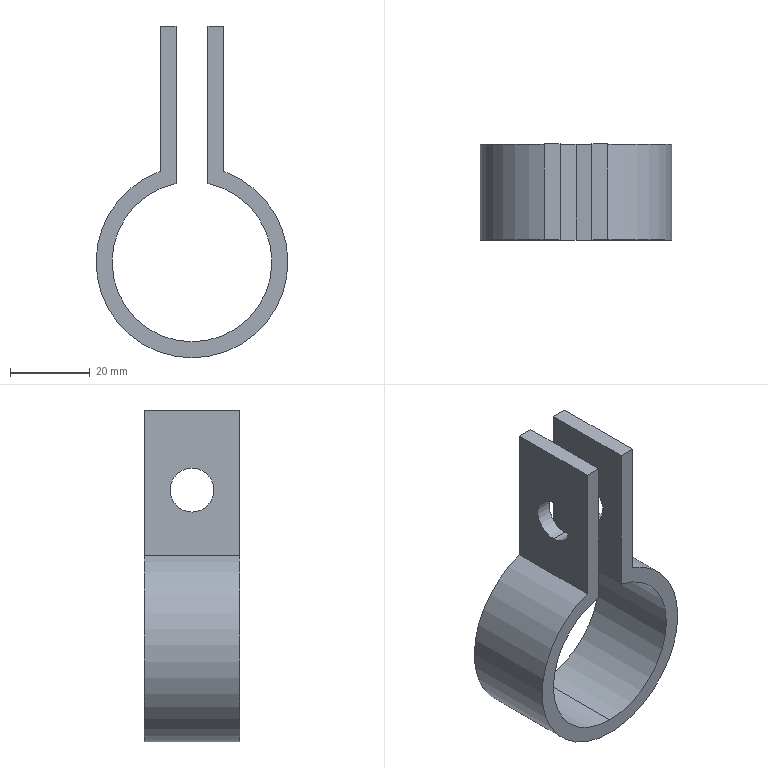Part | SolidWorks | features Extrusion 1, ICE 1 | 1 solid | 16 faces | box 48 x 24 x 83 mm | volume 18610 mm3 | cylinder 8 | plane 8 | commonest cylinder face diameters 11 x4 40 x2 48 x2
STEP:
#1=CARTESIAN_POINT('',(-8.,0.,44.5));
#2=VERTEX_POINT('',#1);
#3=CARTESIAN_POINT('',(-8.,0.,33.5));
#4=VERTEX_POINT('',#3);
#5=CARTESIAN_POINT('',(-8.,0.,39.));
#6=DIRECTION('',(1.,0.,0.));
#7=DIRECTION('',(0.,0.,-1.));
#8=AXIS2_PLACEMENT_3D('',#5,#6,#7);
#9=CIRCLE('',#8,5.5);
#10=EDGE_CURVE('',#2,#4,#9,.T.);
#11=ORIENTED_EDGE('',*,*,#10,.F.);
#12=CARTESIAN_POINT('',(-4.,0.,44.5));
#13=VERTEX_POINT('',#12);
#14=CARTESIAN_POINT('',(-24.,0.,44.5));
#15=DIRECTION('',(1.,0.,0.));
#16=VECTOR('',#15,1000.);
#17=LINE('',#14,#16);
#18=EDGE_CURVE('',#2,#13,#17,.T.);
#19=ORIENTED_EDGE('',*,*,#18,.T.);
#20=CARTESIAN_POINT('',(-4.,0.,33.5));
#21=VERTEX_POINT('',#20);
#22=CARTESIAN_POINT('',(-4.,0.,39.));
#23=DIRECTION('',(-1.,0.,0.));
#24=DIRECTION('',(0.,0.,1.));
#25=AXIS2_PLACEMENT_3D('',#22,#23,#24);
#26=CIRCLE('',#25,5.5);
#27=EDGE_CURVE('',#21,#13,#26,.T.);
#28=ORIENTED_EDGE('',*,*,#27,.F.);
#29=CARTESIAN_POINT('',(-24.,0.,33.5));
#30=DIRECTION('',(1.,0.,0.));
#31=VECTOR('',#30,1000.);
#32=LINE('',#29,#31);
#33=EDGE_CURVE('',#4,#21,#32,.T.);
#34=ORIENTED_EDGE('',*,*,#33,.F.);
#35=EDGE_LOOP('',(#11,#19,#28,#34));
#36=FACE_OUTER_BOUND('',#35,.T.);
#37=CARTESIAN_POINT('',(-24.,0.,39.));
#38=DIRECTION('',(1.,0.,0.));
#39=DIRECTION('',(0.,0.,-1.));
#40=AXIS2_PLACEMENT_3D('',#37,#38,#39);
#41=CYLINDRICAL_SURFACE('',#40,5.5);
#42=ADVANCED_FACE('',(#36),#41,.F.);
#43=CARTESIAN_POINT('',(4.,0.,44.5));
#44=VERTEX_POINT('',#43);
#45=CARTESIAN_POINT('',(4.,0.,33.5));
#46=VERTEX_POINT('',#45);
#47=CARTESIAN_POINT('',(4.,0.,39.));
#48=DIRECTION('',(1.,0.,0.));
#49=DIRECTION('',(0.,0.,-1.));
#50=AXIS2_PLACEMENT_3D('',#47,#48,#49);
#51=CIRCLE('',#50,5.5);
#52=EDGE_CURVE('',#44,#46,#51,.T.);
#53=ORIENTED_EDGE('',*,*,#52,.F.);
#54=CARTESIAN_POINT('',(8.,0.,44.5));
#55=VERTEX_POINT('',#54);
#56=CARTESIAN_POINT('',(-24.,0.,44.5));
#57=DIRECTION('',(1.,0.,0.));
#58=VECTOR('',#57,1000.);
#59=LINE('',#56,#58);
#60=EDGE_CURVE('',#44,#55,#59,.T.);
#61=ORIENTED_EDGE('',*,*,#60,.T.);
#62=CARTESIAN_POINT('',(8.,0.,33.5));
#63=VERTEX_POINT('',#62);
#64=CARTESIAN_POINT('',(8.,0.,39.));
#65=DIRECTION('',(-1.,0.,0.));
#66=DIRECTION('',(0.,0.,1.));
#67=AXIS2_PLACEMENT_3D('',#64,#65,#66);
#68=CIRCLE('',#67,5.5);
#69=EDGE_CURVE('',#63,#55,#68,.T.);
#70=ORIENTED_EDGE('',*,*,#69,.F.);
#71=CARTESIAN_POINT('',(-24.,0.,33.5));
#72=DIRECTION('',(1.,0.,0.));
#73=VECTOR('',#72,1000.);
#74=LINE('',#71,#73);
#75=EDGE_CURVE('',#46,#63,#74,.T.);
#76=ORIENTED_EDGE('',*,*,#75,.F.);
#77=EDGE_LOOP('',(#53,#61,#70,#76));
#78=FACE_OUTER_BOUND('',#77,.T.);
#79=CARTESIAN_POINT('',(-24.,0.,39.));
#80=DIRECTION('',(1.,0.,0.));
#81=DIRECTION('',(0.,0.,-1.));
#82=AXIS2_PLACEMENT_3D('',#79,#80,#81);
#83=CYLINDRICAL_SURFACE('',#82,5.5);
#84=ADVANCED_FACE('',(#78),#83,.F.);
#85=CARTESIAN_POINT('',(0.,12.,-20.));
#86=VERTEX_POINT('',#85);
#87=CARTESIAN_POINT('',(4.,12.,19.596));
#88=VERTEX_POINT('',#87);
#89=CARTESIAN_POINT('',(0.,12.,0.));
#90=DIRECTION('',(0.,-1.,0.));
#91=DIRECTION('',(0.,0.,1.));
#92=AXIS2_PLACEMENT_3D('',#89,#90,#91);
#93=CIRCLE('',#92,20.);
#94=EDGE_CURVE('',#86,#88,#93,.T.);
#95=ORIENTED_EDGE('',*,*,#94,.F.);
#96=CARTESIAN_POINT('',(0.,-12.,-20.));
#97=VERTEX_POINT('',#96);
#98=CARTESIAN_POINT('',(0.,12.,-20.));
#99=DIRECTION('',(0.,-1.,0.));
#100=VECTOR('',#99,1000.);
#101=LINE('',#98,#100);
#102=EDGE_CURVE('',#86,#97,#101,.T.);
#103=ORIENTED_EDGE('',*,*,#102,.T.);
#104=CARTESIAN_POINT('',(4.,-12.,19.596));
#105=VERTEX_POINT('',#104);
#106=CARTESIAN_POINT('',(0.,-12.,0.));
#107=DIRECTION('',(0.,-1.,0.));
#108=DIRECTION('',(0.,0.,1.));
#109=AXIS2_PLACEMENT_3D('',#106,#107,#108);
#110=CIRCLE('',#109,20.);
#111=EDGE_CURVE('',#97,#105,#110,.T.);
#112=ORIENTED_EDGE('',*,*,#111,.T.);
#113=CARTESIAN_POINT('',(4.,12.,19.596));
#114=DIRECTION('',(0.,-1.,0.));
#115=VECTOR('',#114,1000.);
#116=LINE('',#113,#115);
#117=EDGE_CURVE('',#88,#105,#116,.T.);
#118=ORIENTED_EDGE('',*,*,#117,.F.);
#119=EDGE_LOOP('',(#95,#103,#112,#118));
#120=FACE_OUTER_BOUND('',#119,.T.);
#121=CARTESIAN_POINT('',(0.,12.,0.));
#122=DIRECTION('',(0.,-1.,0.));
#123=DIRECTION('',(0.,0.,-1.));
#124=AXIS2_PLACEMENT_3D('',#121,#122,#123);
#125=CYLINDRICAL_SURFACE('',#124,20.);
#126=ADVANCED_FACE('',(#120),#125,.F.);
#127=CARTESIAN_POINT('',(0.,12.,-24.));
#128=VERTEX_POINT('',#127);
#129=CARTESIAN_POINT('',(-8.,12.,22.627));
#130=VERTEX_POINT('',#129);
#131=CARTESIAN_POINT('',(0.,12.,0.));
#132=DIRECTION('',(0.,1.,0.));
#133=DIRECTION('',(0.,0.,1.));
#134=AXIS2_PLACEMENT_3D('',#131,#132,#133);
#135=CIRCLE('',#134,24.);
#136=EDGE_CURVE('',#128,#130,#135,.T.);
#137=ORIENTED_EDGE('',*,*,#136,.F.);
#138=CARTESIAN_POINT('',(0.,-12.,-24.));
#139=VERTEX_POINT('',#138);
#140=CARTESIAN_POINT('',(0.,12.,-24.));
#141=DIRECTION('',(0.,-1.,0.));
#142=VECTOR('',#141,1000.);
#143=LINE('',#140,#142);
#144=EDGE_CURVE('',#128,#139,#143,.T.);
#145=ORIENTED_EDGE('',*,*,#144,.T.);
#146=CARTESIAN_POINT('',(-8.,-12.,22.627));
#147=VERTEX_POINT('',#146);
#148=CARTESIAN_POINT('',(0.,-12.,0.));
#149=DIRECTION('',(0.,1.,0.));
#150=DIRECTION('',(0.,0.,1.));
#151=AXIS2_PLACEMENT_3D('',#148,#149,#150);
#152=CIRCLE('',#151,24.);
#153=EDGE_CURVE('',#139,#147,#152,.T.);
#154=ORIENTED_EDGE('',*,*,#153,.T.);
#155=CARTESIAN_POINT('',(-8.,12.,22.627));
#156=DIRECTION('',(0.,-1.,0.));
#157=VECTOR('',#156,1000.);
#158=LINE('',#155,#157);
#159=EDGE_CURVE('',#130,#147,#158,.T.);
#160=ORIENTED_EDGE('',*,*,#159,.F.);
#161=EDGE_LOOP('',(#137,#145,#154,#160));
#162=FACE_OUTER_BOUND('',#161,.T.);
#163=CARTESIAN_POINT('',(0.,12.,0.));
#164=DIRECTION('',(0.,-1.,0.));
#165=DIRECTION('',(0.,0.,-1.));
#166=AXIS2_PLACEMENT_3D('',#163,#164,#165);
#167=CYLINDRICAL_SURFACE('',#166,24.);
#168=ADVANCED_FACE('',(#162),#167,.T.);
#169=ORIENTED_EDGE('',*,*,#69,.T.);
#170=CARTESIAN_POINT('',(8.,0.,39.));
#171=DIRECTION('',(-1.,0.,0.));
#172=DIRECTION('',(0.,0.,1.));
#173=AXIS2_PLACEMENT_3D('',#170,#171,#172);
#174=CIRCLE('',#173,5.5);
#175=EDGE_CURVE('',#55,#63,#174,.T.);
#176=ORIENTED_EDGE('',*,*,#175,.T.);
#177=EDGE_LOOP('',(#169,#176));
#178=FACE_BOUND('',#177,.T.);
#179=CARTESIAN_POINT('',(8.,-12.,59.));
#180=VERTEX_POINT('',#179);
#181=CARTESIAN_POINT('',(8.,-12.,22.627));
#182=VERTEX_POINT('',#181);
#183=CARTESIAN_POINT('',(8.,-12.,22.627));
#184=DIRECTION('',(0.,0.,-1.));
#185=VECTOR('',#184,1000.);
#186=LINE('',#183,#185);
#187=EDGE_CURVE('',#180,#182,#186,.T.);
#188=ORIENTED_EDGE('',*,*,#187,.T.);
#189=CARTESIAN_POINT('',(8.,12.,22.627));
#190=VERTEX_POINT('',#189);
#191=CARTESIAN_POINT('',(8.,12.,22.627));
#192=DIRECTION('',(0.,-1.,0.));
#193=VECTOR('',#192,1000.);
#194=LINE('',#191,#193);
#195=EDGE_CURVE('',#190,#182,#194,.T.);
#196=ORIENTED_EDGE('',*,*,#195,.F.);
#197=CARTESIAN_POINT('',(8.,12.,59.));
#198=VERTEX_POINT('',#197);
#199=CARTESIAN_POINT('',(8.,12.,22.627));
#200=DIRECTION('',(0.,0.,-1.));
#201=VECTOR('',#200,1000.);
#202=LINE('',#199,#201);
#203=EDGE_CURVE('',#198,#190,#202,.T.);
#204=ORIENTED_EDGE('',*,*,#203,.F.);
#205=CARTESIAN_POINT('',(8.,12.,59.));
#206=DIRECTION('',(0.,-1.,0.));
#207=VECTOR('',#206,1000.);
#208=LINE('',#205,#207);
#209=EDGE_CURVE('',#198,#180,#208,.T.);
#210=ORIENTED_EDGE('',*,*,#209,.T.);
#211=EDGE_LOOP('',(#188,#196,#204,#210));
#212=FACE_OUTER_BOUND('',#211,.T.);
#213=CARTESIAN_POINT('',(8.,12.,22.627));
#214=DIRECTION('',(-1.,0.,0.));
#215=DIRECTION('',(0.,0.,1.));
#216=AXIS2_PLACEMENT_3D('',#213,#214,#215);
#217=PLANE('',#216);
#218=ADVANCED_FACE('',(#178,#212),#217,.F.);
#219=ORIENTED_EDGE('',*,*,#144,.F.);
#220=CARTESIAN_POINT('',(0.,12.,0.));
#221=DIRECTION('',(0.,1.,0.));
#222=DIRECTION('',(0.,0.,1.));
#223=AXIS2_PLACEMENT_3D('',#220,#221,#222);
#224=CIRCLE('',#223,24.);
#225=EDGE_CURVE('',#190,#128,#224,.T.);
#226=ORIENTED_EDGE('',*,*,#225,.F.);
#227=ORIENTED_EDGE('',*,*,#195,.T.);
#228=CARTESIAN_POINT('',(0.,-12.,0.));
#229=DIRECTION('',(0.,1.,0.));
#230=DIRECTION('',(0.,0.,1.));
#231=AXIS2_PLACEMENT_3D('',#228,#229,#230);
#232=CIRCLE('',#231,24.);
#233=EDGE_CURVE('',#182,#139,#232,.T.);
#234=ORIENTED_EDGE('',*,*,#233,.T.);
#235=EDGE_LOOP('',(#219,#226,#227,#234));
#236=FACE_OUTER_BOUND('',#235,.T.);
#237=CARTESIAN_POINT('',(0.,12.,0.));
#238=DIRECTION('',(0.,-1.,0.));
#239=DIRECTION('',(0.,0.,-1.));
#240=AXIS2_PLACEMENT_3D('',#237,#238,#239);
#241=CYLINDRICAL_SURFACE('',#240,24.);
#242=ADVANCED_FACE('',(#236),#241,.T.);
#243=CARTESIAN_POINT('',(-8.,0.,39.));
#244=DIRECTION('',(1.,0.,0.));
#245=DIRECTION('',(0.,0.,-1.));
#246=AXIS2_PLACEMENT_3D('',#243,#244,#245);
#247=CIRCLE('',#246,5.5);
#248=EDGE_CURVE('',#4,#2,#247,.T.);
#249=ORIENTED_EDGE('',*,*,#248,.T.);
#250=ORIENTED_EDGE('',*,*,#10,.T.);
#251=EDGE_LOOP('',(#249,#250));
#252=FACE_BOUND('',#251,.T.);
#253=CARTESIAN_POINT('',(-8.,-12.,59.));
#254=VERTEX_POINT('',#253);
#255=CARTESIAN_POINT('',(-8.,-12.,22.627));
#256=DIRECTION('',(0.,0.,1.));
#257=VECTOR('',#256,1000.);
#258=LINE('',#255,#257);
#259=EDGE_CURVE('',#147,#254,#258,.T.);
#260=ORIENTED_EDGE('',*,*,#259,.T.);
#261=CARTESIAN_POINT('',(-8.,12.,59.));
#262=VERTEX_POINT('',#261);
#263=CARTESIAN_POINT('',(-8.,12.,59.));
#264=DIRECTION('',(0.,-1.,0.));
#265=VECTOR('',#264,1000.);
#266=LINE('',#263,#265);
#267=EDGE_CURVE('',#262,#254,#266,.T.);
#268=ORIENTED_EDGE('',*,*,#267,.F.);
#269=CARTESIAN_POINT('',(-8.,12.,22.627));
#270=DIRECTION('',(0.,0.,1.));
#271=VECTOR('',#270,1000.);
#272=LINE('',#269,#271);
#273=EDGE_CURVE('',#130,#262,#272,.T.);
#274=ORIENTED_EDGE('',*,*,#273,.F.);
#275=ORIENTED_EDGE('',*,*,#159,.T.);
#276=EDGE_LOOP('',(#260,#268,#274,#275));
#277=FACE_OUTER_BOUND('',#276,.T.);
#278=CARTESIAN_POINT('',(-8.,12.,22.627));
#279=DIRECTION('',(1.,0.,0.));
#280=DIRECTION('',(0.,0.,-1.));
#281=AXIS2_PLACEMENT_3D('',#278,#279,#280);
#282=PLANE('',#281);
#283=ADVANCED_FACE('',(#252,#277),#282,.F.);
#284=CARTESIAN_POINT('',(-4.,-12.,59.));
#285=VERTEX_POINT('',#284);
#286=CARTESIAN_POINT('',(-8.,-12.,59.));
#287=DIRECTION('',(1.,0.,0.));
#288=VECTOR('',#287,1000.);
#289=LINE('',#286,#288);
#290=EDGE_CURVE('',#254,#285,#289,.T.);
#291=ORIENTED_EDGE('',*,*,#290,.T.);
#292=CARTESIAN_POINT('',(-4.,12.,59.));
#293=VERTEX_POINT('',#292);
#294=CARTESIAN_POINT('',(-4.,12.,59.));
#295=DIRECTION('',(0.,-1.,0.));
#296=VECTOR('',#295,1000.);
#297=LINE('',#294,#296);
#298=EDGE_CURVE('',#293,#285,#297,.T.);
#299=ORIENTED_EDGE('',*,*,#298,.F.);
#300=CARTESIAN_POINT('',(-8.,12.,59.));
#301=DIRECTION('',(1.,0.,0.));
#302=VECTOR('',#301,1000.);
#303=LINE('',#300,#302);
#304=EDGE_CURVE('',#262,#293,#303,.T.);
#305=ORIENTED_EDGE('',*,*,#304,.F.);
#306=ORIENTED_EDGE('',*,*,#267,.T.);
#307=EDGE_LOOP('',(#291,#299,#305,#306));
#308=FACE_OUTER_BOUND('',#307,.T.);
#309=CARTESIAN_POINT('',(-8.,12.,59.));
#310=DIRECTION('',(0.,0.,-1.));
#311=DIRECTION('',(-1.,0.,0.));
#312=AXIS2_PLACEMENT_3D('',#309,#310,#311);
#313=PLANE('',#312);
#314=ADVANCED_FACE('',(#308),#313,.F.);
#315=ORIENTED_EDGE('',*,*,#27,.T.);
#316=CARTESIAN_POINT('',(-4.,0.,39.));
#317=DIRECTION('',(-1.,0.,0.));
#318=DIRECTION('',(0.,0.,1.));
#319=AXIS2_PLACEMENT_3D('',#316,#317,#318);
#320=CIRCLE('',#319,5.5);
#321=EDGE_CURVE('',#13,#21,#320,.T.);
#322=ORIENTED_EDGE('',*,*,#321,.T.);
#323=EDGE_LOOP('',(#315,#322));
#324=FACE_BOUND('',#323,.T.);
#325=CARTESIAN_POINT('',(-4.,-12.,19.596));
#326=VERTEX_POINT('',#325);
#327=CARTESIAN_POINT('',(-4.,-12.,19.596));
#328=DIRECTION('',(0.,0.,-1.));
#329=VECTOR('',#328,1000.);
#330=LINE('',#327,#329);
#331=EDGE_CURVE('',#285,#326,#330,.T.);
#332=ORIENTED_EDGE('',*,*,#331,.T.);
#333=CARTESIAN_POINT('',(-4.,12.,19.596));
#334=VERTEX_POINT('',#333);
#335=CARTESIAN_POINT('',(-4.,12.,19.596));
#336=DIRECTION('',(0.,-1.,0.));
#337=VECTOR('',#336,1000.);
#338=LINE('',#335,#337);
#339=EDGE_CURVE('',#334,#326,#338,.T.);
#340=ORIENTED_EDGE('',*,*,#339,.F.);
#341=CARTESIAN_POINT('',(-4.,12.,19.596));
#342=DIRECTION('',(0.,0.,-1.));
#343=VECTOR('',#342,1000.);
#344=LINE('',#341,#343);
#345=EDGE_CURVE('',#293,#334,#344,.T.);
#346=ORIENTED_EDGE('',*,*,#345,.F.);
#347=ORIENTED_EDGE('',*,*,#298,.T.);
#348=EDGE_LOOP('',(#332,#340,#346,#347));
#349=FACE_OUTER_BOUND('',#348,.T.);
#350=CARTESIAN_POINT('',(-4.,12.,19.596));
#351=DIRECTION('',(-1.,0.,0.));
#352=DIRECTION('',(0.,0.,1.));
#353=AXIS2_PLACEMENT_3D('',#350,#351,#352);
#354=PLANE('',#353);
#355=ADVANCED_FACE('',(#324,#349),#354,.F.);
#356=ORIENTED_EDGE('',*,*,#102,.F.);
#357=CARTESIAN_POINT('',(0.,12.,0.));
#358=DIRECTION('',(0.,-1.,0.));
#359=DIRECTION('',(0.,0.,1.));
#360=AXIS2_PLACEMENT_3D('',#357,#358,#359);
#361=CIRCLE('',#360,20.);
#362=EDGE_CURVE('',#334,#86,#361,.T.);
#363=ORIENTED_EDGE('',*,*,#362,.F.);
#364=ORIENTED_EDGE('',*,*,#339,.T.);
#365=CARTESIAN_POINT('',(0.,-12.,0.));
#366=DIRECTION('',(0.,-1.,0.));
#367=DIRECTION('',(0.,0.,1.));
#368=AXIS2_PLACEMENT_3D('',#365,#366,#367);
#369=CIRCLE('',#368,20.);
#370=EDGE_CURVE('',#326,#97,#369,.T.);
#371=ORIENTED_EDGE('',*,*,#370,.T.);
#372=EDGE_LOOP('',(#356,#363,#364,#371));
#373=FACE_OUTER_BOUND('',#372,.T.);
#374=CARTESIAN_POINT('',(0.,12.,0.));
#375=DIRECTION('',(0.,-1.,0.));
#376=DIRECTION('',(0.,0.,-1.));
#377=AXIS2_PLACEMENT_3D('',#374,#375,#376);
#378=CYLINDRICAL_SURFACE('',#377,20.);
#379=ADVANCED_FACE('',(#373),#378,.F.);
#380=CARTESIAN_POINT('',(4.,0.,39.));
#381=DIRECTION('',(1.,0.,0.));
#382=DIRECTION('',(0.,0.,-1.));
#383=AXIS2_PLACEMENT_3D('',#380,#381,#382);
#384=CIRCLE('',#383,5.5);
#385=EDGE_CURVE('',#46,#44,#384,.T.);
#386=ORIENTED_EDGE('',*,*,#385,.T.);
#387=ORIENTED_EDGE('',*,*,#52,.T.);
#388=EDGE_LOOP('',(#386,#387));
#389=FACE_BOUND('',#388,.T.);
#390=CARTESIAN_POINT('',(4.,-12.,59.));
#391=VERTEX_POINT('',#390);
#392=CARTESIAN_POINT('',(4.,-12.,19.596));
#393=DIRECTION('',(0.,0.,1.));
#394=VECTOR('',#393,1000.);
#395=LINE('',#392,#394);
#396=EDGE_CURVE('',#105,#391,#395,.T.);
#397=ORIENTED_EDGE('',*,*,#396,.T.);
#398=CARTESIAN_POINT('',(4.,12.,59.));
#399=VERTEX_POINT('',#398);
#400=CARTESIAN_POINT('',(4.,12.,59.));
#401=DIRECTION('',(0.,-1.,0.));
#402=VECTOR('',#401,1000.);
#403=LINE('',#400,#402);
#404=EDGE_CURVE('',#399,#391,#403,.T.);
#405=ORIENTED_EDGE('',*,*,#404,.F.);
#406=CARTESIAN_POINT('',(4.,12.,19.596));
#407=DIRECTION('',(0.,0.,1.));
#408=VECTOR('',#407,1000.);
#409=LINE('',#406,#408);
#410=EDGE_CURVE('',#88,#399,#409,.T.);
#411=ORIENTED_EDGE('',*,*,#410,.F.);
#412=ORIENTED_EDGE('',*,*,#117,.T.);
#413=EDGE_LOOP('',(#397,#405,#411,#412));
#414=FACE_OUTER_BOUND('',#413,.T.);
#415=CARTESIAN_POINT('',(4.,12.,19.596));
#416=DIRECTION('',(1.,0.,0.));
#417=DIRECTION('',(0.,0.,-1.));
#418=AXIS2_PLACEMENT_3D('',#415,#416,#417);
#419=PLANE('',#418);
#420=ADVANCED_FACE('',(#389,#414),#419,.F.);
#421=CARTESIAN_POINT('',(8.,-12.,59.));
#422=DIRECTION('',(1.,0.,0.));
#423=VECTOR('',#422,1000.);
#424=LINE('',#421,#423);
#425=EDGE_CURVE('',#391,#180,#424,.T.);
#426=ORIENTED_EDGE('',*,*,#425,.T.);
#427=ORIENTED_EDGE('',*,*,#209,.F.);
#428=CARTESIAN_POINT('',(8.,12.,59.));
#429=DIRECTION('',(1.,0.,0.));
#430=VECTOR('',#429,1000.);
#431=LINE('',#428,#430);
#432=EDGE_CURVE('',#399,#198,#431,.T.);
#433=ORIENTED_EDGE('',*,*,#432,.F.);
#434=ORIENTED_EDGE('',*,*,#404,.T.);
#435=EDGE_LOOP('',(#426,#427,#433,#434));
#436=FACE_OUTER_BOUND('',#435,.T.);
#437=CARTESIAN_POINT('',(8.,12.,59.));
#438=DIRECTION('',(0.,0.,-1.));
#439=DIRECTION('',(-1.,0.,0.));
#440=AXIS2_PLACEMENT_3D('',#437,#438,#439);
#441=PLANE('',#440);
#442=ADVANCED_FACE('',(#436),#441,.F.);
#443=ORIENTED_EDGE('',*,*,#203,.T.);
#444=ORIENTED_EDGE('',*,*,#225,.T.);
#445=ORIENTED_EDGE('',*,*,#136,.T.);
#446=ORIENTED_EDGE('',*,*,#273,.T.);
#447=ORIENTED_EDGE('',*,*,#304,.T.);
#448=ORIENTED_EDGE('',*,*,#345,.T.);
#449=ORIENTED_EDGE('',*,*,#362,.T.);
#450=ORIENTED_EDGE('',*,*,#94,.T.);
#451=ORIENTED_EDGE('',*,*,#410,.T.);
#452=ORIENTED_EDGE('',*,*,#432,.T.);
#453=EDGE_LOOP('',(#443,#444,#445,#446,#447,#448,#449,#450,#451,#452));
#454=FACE_OUTER_BOUND('',#453,.T.);
#455=CARTESIAN_POINT('',(0.,12.,0.));
#456=DIRECTION('',(0.,1.,0.));
#457=DIRECTION('',(0.,0.,1.));
#458=AXIS2_PLACEMENT_3D('',#455,#456,#457);
#459=PLANE('',#458);
#460=ADVANCED_FACE('',(#454),#459,.T.);
#461=ORIENTED_EDGE('',*,*,#187,.F.);
#462=ORIENTED_EDGE('',*,*,#425,.F.);
#463=ORIENTED_EDGE('',*,*,#396,.F.);
#464=ORIENTED_EDGE('',*,*,#111,.F.);
#465=ORIENTED_EDGE('',*,*,#370,.F.);
#466=ORIENTED_EDGE('',*,*,#331,.F.);
#467=ORIENTED_EDGE('',*,*,#290,.F.);
#468=ORIENTED_EDGE('',*,*,#259,.F.);
#469=ORIENTED_EDGE('',*,*,#153,.F.);
#470=ORIENTED_EDGE('',*,*,#233,.F.);
#471=EDGE_LOOP('',(#461,#462,#463,#464,#465,#466,#467,#468,#469,#470));
#472=FACE_OUTER_BOUND('',#471,.T.);
#473=CARTESIAN_POINT('',(0.,-12.,0.));
#474=DIRECTION('',(0.,1.,0.));
#475=DIRECTION('',(0.,0.,1.));
#476=AXIS2_PLACEMENT_3D('',#473,#474,#475);
#477=PLANE('',#476);
#478=ADVANCED_FACE('',(#472),#477,.F.);
#479=ORIENTED_EDGE('',*,*,#60,.F.);
#480=ORIENTED_EDGE('',*,*,#385,.F.);
#481=ORIENTED_EDGE('',*,*,#75,.T.);
#482=ORIENTED_EDGE('',*,*,#175,.F.);
#483=EDGE_LOOP('',(#479,#480,#481,#482));
#484=FACE_OUTER_BOUND('',#483,.T.);
#485=CARTESIAN_POINT('',(-24.,0.,39.));
#486=DIRECTION('',(1.,0.,0.));
#487=DIRECTION('',(0.,0.,-1.));
#488=AXIS2_PLACEMENT_3D('',#485,#486,#487);
#489=CYLINDRICAL_SURFACE('',#488,5.5);
#490=ADVANCED_FACE('',(#484),#489,.F.);
#491=ORIENTED_EDGE('',*,*,#18,.F.);
#492=ORIENTED_EDGE('',*,*,#248,.F.);
#493=ORIENTED_EDGE('',*,*,#33,.T.);
#494=ORIENTED_EDGE('',*,*,#321,.F.);
#495=EDGE_LOOP('',(#491,#492,#493,#494));
#496=FACE_OUTER_BOUND('',#495,.T.);
#497=CARTESIAN_POINT('',(-24.,0.,39.));
#498=DIRECTION('',(1.,0.,0.));
#499=DIRECTION('',(0.,0.,-1.));
#500=AXIS2_PLACEMENT_3D('',#497,#498,#499);
#501=CYLINDRICAL_SURFACE('',#500,5.5);
#502=ADVANCED_FACE('',(#496),#501,.F.);
#503=CLOSED_SHELL('',(#42,#84,#126,#168,#218,#242,#283,#314,#355,#379,#420,#442,#460,#478,#490,#502));
#504=MANIFOLD_SOLID_BREP('',#503);
#505=CARTESIAN_POINT('',(0.,0.,0.));
#506=DIRECTION('',(0.,0.,1.));
#507=DIRECTION('',(1.,0.,0.));
#508=AXIS2_PLACEMENT_3D('',#505,#506,#507);
#509=(LENGTH_UNIT()NAMED_UNIT(*)SI_UNIT(.MILLI.,.METRE.));
#510=UNCERTAINTY_MEASURE_WITH_UNIT(LENGTH_MEASURE(0.00001),#509,'','');
#511=(NAMED_UNIT(*)PLANE_ANGLE_UNIT()SI_UNIT($,.RADIAN.));
#512=(NAMED_UNIT(*)SI_UNIT($,.STERADIAN.)SOLID_ANGLE_UNIT());
#513=(GEOMETRIC_REPRESENTATION_CONTEXT(3)GLOBAL_UNCERTAINTY_ASSIGNED_CONTEXT((#510))GLOBAL_UNIT_ASSIGNED_CONTEXT((#509,#511,#512))REPRESENTATION_CONTEXT('',''));
#514=ADVANCED_BREP_SHAPE_REPRESENTATION('',(#504,#508),#513);